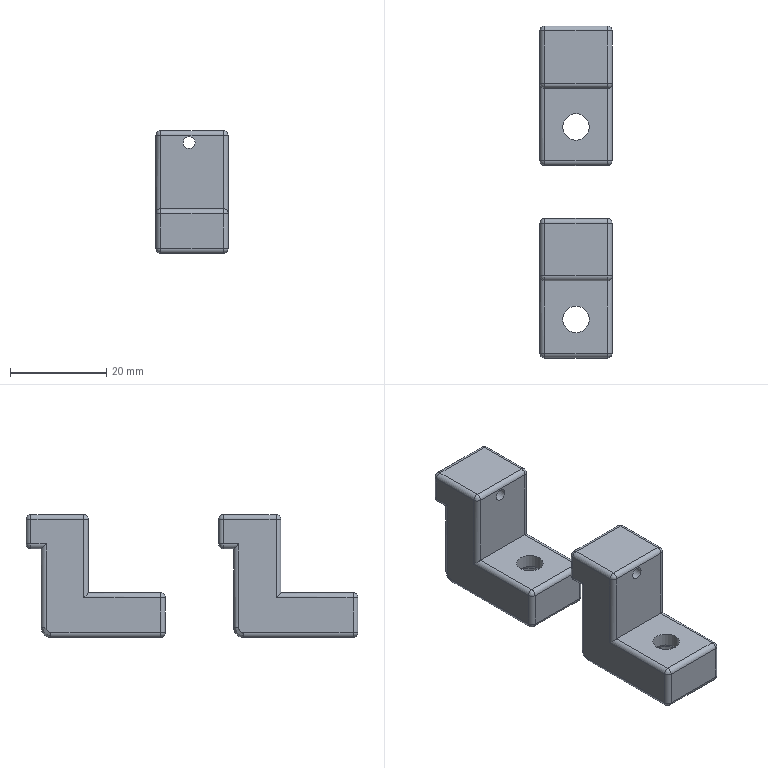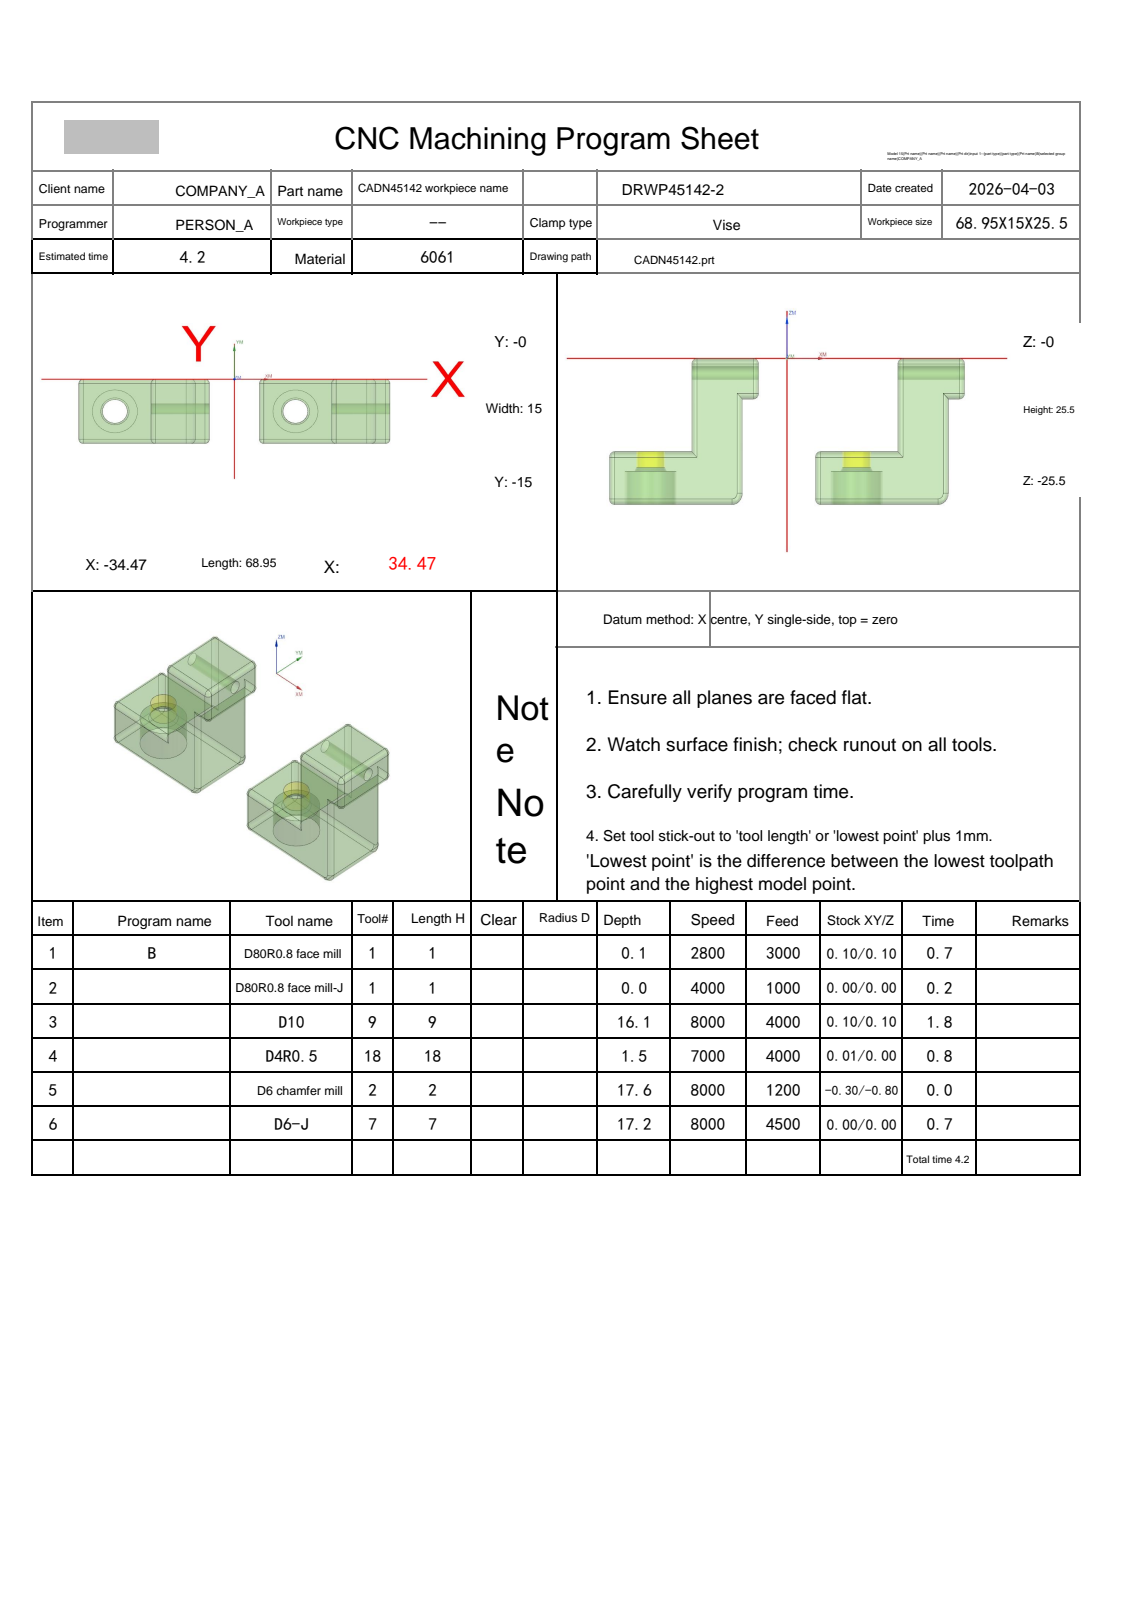NC program | NX | posted by the shop | part box 15 x 68.95 x 25.5 mm
Lines 8095 to 8513 of 8513:
N5 T02 M06
(D6 chamfer mill  D=6. R=0. H=02 ce=-0.30 di=-0.80)
G00 G90 G54 X12.878 Y-7.564 M03 S8000
G43 H02 Z20.
M08
Z-17.15
G01 Z-17.65 F1200.
X12.025 Y-7.65
G03 X13.525 Y-9.15 I1.5 J0.0
X15.175 Y-7.5 I0.0 J1.65
X13.525 Y-5.85 I-1.65 J0.0
X11.875 Y-7.5 I0.0 J-1.65
X13.525 Y-9.15 I1.65 J0.0
X15.025 Y-7.65 I0.0 J1.5
G01 X14.172 Y-7.564
Z-17.15
G00 Z20.
X-27.122
Z-17.15
G01 Z-17.65
X-27.975 Y-7.65
G03 X-26.475 Y-9.15 I1.5 J0.0
X-24.825 Y-7.5 I0.0 J1.65
X-26.475 Y-5.85 I-1.65 J0.0
X-28.125 Y-7.5 I0.0 J-1.65
X-26.475 Y-9.15 I1.65 J0.0
X-24.975 Y-7.65 I0.0 J1.5
G01 X-25.828 Y-7.564
Z-17.15
G00 Z20.
G91 G28 Z0.0
M05
M09
G91 G28 Z0.0
M01
N6 T07 M06
(D6-J  D=6. R=0. H=07 ce=0.40 di=0.00)
G00 G90 G54 X2.325 Y-8.7 M03 S7000
G43 H07 Z14.
M08
Z-14.75
G01 Z-16.25 F1500.
X4.725
G03 X5.925 Y-7.5 I0.0 J1.2
G01 Y-.999
G02 X6.524 Y-.4 I.6 J-.001
G01 X17.526
G02 X18.125 Y-.999 I-.001 J-.6
G01 Y-14.001
G02 X17.526 Y-14.6 I-.6 J.001
G01 X6.524
G02 X5.925 Y-14. I.001 J.6
G01 Y-6.321
G02 X6.192 Y-5.822 I.6 J0.0
G01 X8.713 Y-4.14
G03 X8.953 Y-3.821 I-.333 J.499
G02 X9.524 Y-3.4 I.573 J-.179
G01 X14.526
G02 X15.125 Y-3.999 I-.001 J-.6
G01 Y-11.001
G02 X14.526 Y-11.6 I-.6 J.001
G01 X9.524
G02 X8.925 Y-11.001 I.001 J.6
G01 Y-6.557
G02 X9.465 Y-6.017 I.54 J0.0
G01 X9.482 Y-6.018
X12.06 Y-6.1
X12.07
G02 X12.425 Y-6.459 I-.005 J-.36
G01 Y-8.541
G02 X12.066 Y-8.9 I-.36 J.001
G01 X11.984
G02 X11.625 Y-8.541 I.001 J.36
G01 Y-6.459
G02 X11.682 Y-6.266 I.36 J-.001
X11.984 Y-6.1 I.303 J-.194
G01 X12.066
G02 X12.425 Y-6.454 I-.001 J-.36
G03 X13.625 Y-7.635 I1.2 J.02
G01 X13.645 Y-7.634
Z-14.75
G00 Z14.
X-37.675 Y-8.7
Z-14.75
G01 Z-16.25
X-35.275
G03 X-34.075 Y-7.5 I0.0 J1.2
G01 Y-.999
G02 X-33.476 Y-.4 I.6 J-.001
G01 X-22.474
G02 X-21.875 Y-.999 I-.001 J-.6
G01 Y-14.001
G02 X-22.474 Y-14.6 I-.6 J.001
G01 X-33.476
G02 X-34.075 Y-14. I.001 J.6
G01 Y-4.5
G02 X-33.475 Y-3.9 I.6 J0.0
G01 X-33.45
X-31.527 Y-3.98
X-31.503 Y-3.981
G03 X-30.989 Y-3.69 I0.0 J.6
G02 X-30.476 Y-3.4 I.514 J-.31
G01 X-25.474
G02 X-24.875 Y-3.999 I-.001 J-.6
G01 Y-11.001
G02 X-25.474 Y-11.6 I-.6 J.001
G01 X-30.476
G02 X-31.075 Y-11.001 I.001 J.6
G01 Y-6.557
G02 X-30.535 Y-6.017 I.54 J0.0
G01 X-30.518 Y-6.018
X-27.94 Y-6.1
X-27.93
G02 X-27.575 Y-6.459 I-.005 J-.36
G01 Y-8.541
G02 X-27.934 Y-8.9 I-.36 J.001
G01 X-28.016
G02 X-28.375 Y-8.541 I.001 J.36
G01 Y-6.459
G02 X-28.318 Y-6.266 I.36 J-.001
X-28.016 Y-6.1 I.303 J-.194
G01 X-27.934
G02 X-27.575 Y-6.454 I-.001 J-.36
G03 X-26.375 Y-7.635 I1.2 J.02
G01 X-26.355 Y-7.634
Z-14.75
G00 Z14.
G00 G90 X23.425 Y-19.1 M03 S8000
Z9.
Z-7.125
G01 Z-8.125 F1000.
G41 D07
Y-18.9
G03 X22.525 Y-18. I-.9 J0.0
G02 X18.525 Y-14. I0.0 J4.
G01 Y-1.
G02 X22.525 Y3. I4. J0.0
G03 X23.425 Y3.9 I0.0 J.9
G01 G40 Y4.1
Z-7.125
G00 Z9.
Y-19.1
Z-15.25
G01 Z-16.25
G41 D07
Y-18.9
G03 X22.525 Y-18. I-.9 J0.0
G02 X18.525 Y-14. I0.0 J4.
G01 Y-1.
G02 X22.525 Y3. I4. J0.0
G03 X23.425 Y3.9 I0.0 J.9
G01 G40 Y4.1
Z-15.25
G00 Z9.
X-16.609 Y-19.1
Z-7.125
G01 Z-8.125
G41 D07
Y-18.9
G03 X-17.502 Y-18. I-.9 J0.0
G02 X-21.475 Y-14. I.028 J4.
G01 Y-1.
G02 X-17.502 Y3. I4. J0.0
G03 X-16.609 Y3.9 I-.006 J.9
G01 G40 Y4.1
Z-7.125
G00 Z9.
Y-19.1
Z-15.25
G01 Z-16.25
G41 D07
Y-18.9
G03 X-17.502 Y-18. I-.9 J0.0
G02 X-21.475 Y-14. I.028 J4.
G01 Y-1.
G02 X-17.502 Y3. I4. J0.0
G03 X-16.609 Y3.9 I-.006 J.9
G01 G40 Y4.1
Z-15.25
G00 Z9.
G00 G90 X-19.606 Y-18.754 M03 S7000
Z14.
Z-15.766
G01 Z-16.266 F4500.
G03 X-19.437 Y-18.14 I-1.031 J.614
X-19.909 Y-17.186 I-1.2 J0.0
G01 X-33.475
G02 X-36.661 Y-14. I0.0 J3.187
G01 Y-1.
G02 X-33.475 Y2.187 I3.187 J0.0
G01 X-19.909
X-19.837 Y2.246 Z-16.278
X-19.765 Y2.292 Z-16.291
X-33.475
G03 X-36.767 Y-1. I0.0 J-3.292
G01 Y-14.
G03 X-33.475 Y-17.292 I3.292 J0.0
G01 X-19.765
X-19.691 Y-17.345 Z-16.308
X-19.616 Y-17.39 Z-16.325
X-33.475
G02 X-36.865 Y-14. I0.0 J3.39
G01 Y-1.
G02 X-33.475 Y2.39 I3.39 J0.0
G01 X-19.616
X-19.539 Y2.44 Z-16.347
X-19.462 Y2.483 Z-16.369
X-33.475
G03 X-36.957 Y-1. I0.0 J-3.483
G01 Y-14.
G03 X-33.475 Y-17.482 I3.483 J0.0
G01 X-19.462
X-19.382 Y-17.528 Z-16.395
X-19.302 Y-17.569 Z-16.421
X-33.475
G02 X-37.044 Y-14. I0.0 J3.57
G01 Y-1.
G02 X-33.475 Y2.57 I3.57 J0.0
G01 X-19.302
X-19.218 Y2.612 Z-16.452
X-19.134 Y2.65 Z-16.482
X-33.475
G03 X-37.125 Y-1. I0.0 J-3.65
G01 Y-14.
G03 X-33.475 Y-17.65 I3.65 J0.0
G01 X-19.134
X-19.048 Y-17.689 Z-16.516
X-18.961 Y-17.724 Z-16.55
X-33.475
G02 X-37.199 Y-14. I0.0 J3.724
G01 Y-1.
G02 X-33.475 Y2.724 I3.724 J0.0
G01 X-18.961
X-18.871 Y2.759 Z-16.588
X-18.781 Y2.791 Z-16.626
X-33.475
G03 X-37.266 Y-1. I0.0 J-3.791
G01 Y-14.
G03 X-33.475 Y-17.791 I3.791 J0.0
G01 X-18.781
X-18.689 Y-17.821 Z-16.666
X-18.597 Y-17.85 Z-16.707
X-33.475
G02 X-37.325 Y-14. I0.0 J3.85
G01 Y-1.
G02 X-33.475 Y2.85 I3.85 J0.0
G01 X-18.597
X-18.502 Y2.876 Z-16.751
X-18.408 Y2.9 Z-16.794
X-33.475
G03 X-37.375 Y-1. I0.0 J-3.9
G01 Y-14.
G03 X-33.475 Y-17.9 I3.9 J0.0
G01 X-18.408
X-18.311 Y-17.922 Z-16.84
X-18.215 Y-17.941 Z-16.885
X-33.475
G02 X-37.416 Y-14. I0.0 J3.941
G01 Y-1.
G02 X-33.475 Y2.941 I3.941 J0.0
G01 X-18.215
X-18.121 Y2.958 Z-16.931
X-18.026 Y2.972 Z-16.976
X-33.475
G03 X-37.447 Y-1. I0.0 J-3.972
G01 Y-14.
G03 X-33.475 Y-17.972 I3.972 J0.0
G01 X-18.026
X-17.934 Y-17.983 Z-17.022
X-17.841 Y-17.993 Z-17.068
X-33.475
G02 X-37.468 Y-14. I0.0 J3.993
G01 Y-1.
G02 X-33.475 Y2.993 I3.993 J0.0
G01 X-17.841
X-17.708 Y3.003 Z-17.09
X-17.575 Y3.009 Z-17.113
X-17.442 Y3.01 Z-17.136
X-17.309 Z-17.159
X-17.582 Y3.009
X-17.657 Y3.006
X-33.475
G03 X-37.481 Y-1. I0.0 J-4.006
G01 Y-14.
G03 X-33.475 Y-18.006 I4.006 J0.0
G01 X-17.657
X-17.562 Y-18.009
X-15.974
X-15.828 Y-18.01 Z-17.25
X-33.634 Y-18.007
G02 X-37.483 Y-14.125 I.159 J4.007
G01 X-37.485 Y-14.
Y-1.
X-37.483 Y-.875
G02 X-33.634 Y3.007 I4.008 J-.125
G01 X-33.485 Y3.009
X-17.309 Y3.01
G00 Z14.
X20.394 Y-18.754
Z-15.766
G01 Z-16.266
G03 X20.563 Y-18.14 I-1.031 J.614
X20.091 Y-17.186 I-1.2 J0.0
G01 X6.525
G02 X3.339 Y-14. I0.0 J3.187
G01 Y-1.
G02 X6.525 Y2.187 I3.187 J0.0
G01 X20.091
X20.163 Y2.246 Z-16.278
X20.235 Y2.292 Z-16.291
X6.525
G03 X3.233 Y-1. I0.0 J-3.292
G01 Y-14.
G03 X6.525 Y-17.292 I3.292 J0.0
G01 X20.235
X20.309 Y-17.345 Z-16.308
X20.384 Y-17.39 Z-16.325
X6.525
G02 X3.135 Y-14. I0.0 J3.39
G01 Y-1.
G02 X6.525 Y2.39 I3.39 J0.0
G01 X20.384
X20.461 Y2.44 Z-16.347
X20.538 Y2.483 Z-16.369
X6.525
G03 X3.043 Y-1. I0.0 J-3.483
G01 Y-14.
G03 X6.525 Y-17.482 I3.483 J0.0
G01 X20.538
X20.618 Y-17.528 Z-16.395
X20.698 Y-17.569 Z-16.421
X6.525
G02 X2.956 Y-14. I0.0 J3.57
G01 Y-1.
G02 X6.525 Y2.57 I3.57 J0.0
G01 X20.698
X20.782 Y2.612 Z-16.452
X20.866 Y2.65 Z-16.482
X6.525
G03 X2.875 Y-1. I0.0 J-3.65
G01 Y-14.
G03 X6.525 Y-17.65 I3.65 J0.0
G01 X20.866
X20.952 Y-17.689 Z-16.516
X21.039 Y-17.724 Z-16.55
X6.525
G02 X2.801 Y-14. I0.0 J3.724
G01 Y-1.
G02 X6.525 Y2.724 I3.724 J0.0
G01 X21.039
X21.129 Y2.759 Z-16.588
X21.219 Y2.791 Z-16.626
X6.525
G03 X2.734 Y-1. I0.0 J-3.791
G01 Y-14.
G03 X6.525 Y-17.791 I3.791 J0.0
G01 X21.219
X21.311 Y-17.821 Z-16.666
X21.403 Y-17.85 Z-16.707
X6.525
G02 X2.675 Y-14. I0.0 J3.85
G01 Y-1.
G02 X6.525 Y2.85 I3.85 J0.0
G01 X21.403
X21.498 Y2.876 Z-16.751
X21.592 Y2.9 Z-16.794
X6.525
G03 X2.625 Y-1. I0.0 J-3.9
G01 Y-14.
G03 X6.525 Y-17.9 I3.9 J0.0
G01 X21.592
X21.689 Y-17.922 Z-16.84
X21.785 Y-17.941 Z-16.885
X6.525
G02 X2.584 Y-14. I0.0 J3.941
G01 Y-1.
G02 X6.525 Y2.941 I3.941 J0.0
G01 X21.785
X21.879 Y2.958 Z-16.931
X21.974 Y2.972 Z-16.976
X6.525
G03 X2.553 Y-1. I0.0 J-3.972
G01 Y-14.
G03 X6.525 Y-17.972 I3.972 J0.0
G01 X21.974
X22.097 Y-17.987 Z-17.007
X22.221 Y-17.998 Z-17.037
X22.345 Y-17.993 Z-17.068
X6.525
G02 X2.532 Y-14. I0.0 J3.993
G01 Y-1.
G02 X6.525 Y2.993 I3.993 J0.0
G01 X22.345
X22.517 Y3.01 Z-17.113
X22.69 Z-17.159
X22.435 Y3.006
X6.525
G03 X2.519 Y-1. I0.0 J-4.006
G01 Y-14.
G03 X6.525 Y-18.006 I4.006 J0.0
G01 X22.435
X22.474 Y-18.009
X24.031
X24.166 Y-18.01 Z-17.25
X6.416 Y-18.008
G02 X2.519 Y-14.163 I.109 J4.009
G01 X2.515 Y-14.
Y-1.
X2.519 Y-.837
G02 X6.416 Y3.009 I4.007 J-.163
G01 X6.515
X22.69 Y3.01
G00 Z14.
M05
M09
G91 G28 Z0.0
G91 G28 Y0.0
M30
%